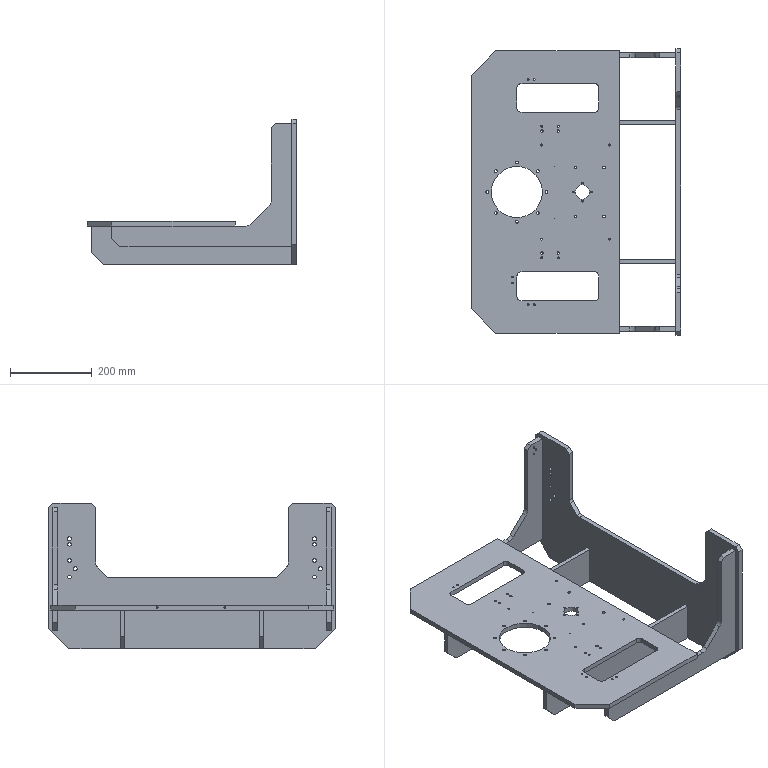Part | NX | features 5003_230_Bracket 2 | 1 solid | 147 faces | box 512 x 700 x 355 mm | volume 6143341 mm3 | cylinder 75 | plane 68 | cone 4 | commonest cylinder face diameters 20 x12 4.2 x11 5 x8 6.8 x8 4.134 x6 9 x6